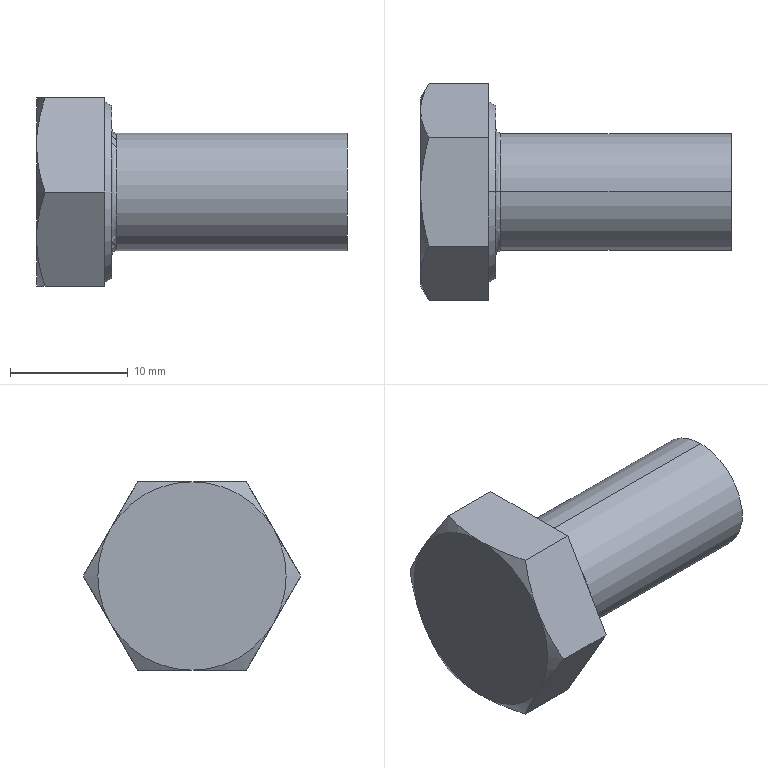Part | SolidWorks | features RevCut 3, Extrusion 1, Fillet 1, LPattern 1, Revolution 1 | 1 solid | 22 faces | box 26.4 x 18.475 x 16 mm | volume 2959 mm3 | plane 10 | cone 8 | torus 2 | cylinder 2 | commonest cylinder face diameters 10 x2
STEP:
#1=CARTESIAN_POINT('',(6.8,0.,5.));
#2=VERTEX_POINT('',#1);
#3=CARTESIAN_POINT('',(6.8,0.,-5.));
#4=VERTEX_POINT('',#3);
#5=CARTESIAN_POINT('',(6.8,0.,0.));
#6=DIRECTION('',(1.,0.,0.));
#7=DIRECTION('',(0.,0.,-1.));
#8=AXIS2_PLACEMENT_3D('',#5,#6,#7);
#9=CIRCLE('',#8,5.);
#10=EDGE_CURVE('',#2,#4,#9,.T.);
#11=ORIENTED_EDGE('',*,*,#10,.F.);
#12=CARTESIAN_POINT('',(6.4,0.,5.4));
#13=VERTEX_POINT('',#12);
#14=CARTESIAN_POINT('',(6.8,0.,5.4));
#15=DIRECTION('',(0.,1.,0.));
#16=DIRECTION('',(0.,0.,1.));
#17=AXIS2_PLACEMENT_3D('',#14,#15,#16);
#18=CIRCLE('',#17,0.4);
#19=EDGE_CURVE('',#2,#13,#18,.T.);
#20=ORIENTED_EDGE('',*,*,#19,.T.);
#21=CARTESIAN_POINT('',(6.4,0.,-5.4));
#22=VERTEX_POINT('',#21);
#23=CARTESIAN_POINT('',(6.4,0.,0.));
#24=DIRECTION('',(-1.,0.,0.));
#25=DIRECTION('',(0.,0.,-1.));
#26=AXIS2_PLACEMENT_3D('',#23,#24,#25);
#27=CIRCLE('',#26,5.4);
#28=EDGE_CURVE('',#22,#13,#27,.T.);
#29=ORIENTED_EDGE('',*,*,#28,.F.);
#30=CARTESIAN_POINT('',(6.8,0.,-5.4));
#31=DIRECTION('',(0.,-1.,0.));
#32=DIRECTION('',(0.,0.,-1.));
#33=AXIS2_PLACEMENT_3D('',#30,#31,#32);
#34=CIRCLE('',#33,0.4);
#35=EDGE_CURVE('',#4,#22,#34,.T.);
#36=ORIENTED_EDGE('',*,*,#35,.F.);
#37=EDGE_LOOP('',(#11,#20,#29,#36));
#38=FACE_OUTER_BOUND('',#37,.T.);
#39=CARTESIAN_POINT('',(6.8,0.,0.));
#40=DIRECTION('',(1.,0.,0.));
#41=DIRECTION('',(0.,0.,-1.));
#42=AXIS2_PLACEMENT_3D('',#39,#40,#41);
#43=TOROIDAL_SURFACE('',#42,5.4,0.4);
#44=ADVANCED_FACE('',(#38),#43,.F.);
#45=CARTESIAN_POINT('',(26.4,0.,5.));
#46=VERTEX_POINT('',#45);
#47=CARTESIAN_POINT('',(26.4,0.,-5.));
#48=VERTEX_POINT('',#47);
#49=CARTESIAN_POINT('',(26.4,0.,0.));
#50=DIRECTION('',(-1.,0.,0.));
#51=DIRECTION('',(0.,0.,1.));
#52=AXIS2_PLACEMENT_3D('',#49,#50,#51);
#53=CIRCLE('',#52,5.);
#54=EDGE_CURVE('',#46,#48,#53,.T.);
#55=ORIENTED_EDGE('',*,*,#54,.T.);
#56=CARTESIAN_POINT('',(0.,0.,-5.));
#57=DIRECTION('',(-1.,0.,0.));
#58=VECTOR('',#57,1000.);
#59=LINE('',#56,#58);
#60=EDGE_CURVE('',#48,#4,#59,.T.);
#61=ORIENTED_EDGE('',*,*,#60,.T.);
#62=CARTESIAN_POINT('',(6.8,0.,0.));
#63=DIRECTION('',(1.,0.,0.));
#64=DIRECTION('',(0.,0.,-1.));
#65=AXIS2_PLACEMENT_3D('',#62,#63,#64);
#66=CIRCLE('',#65,5.);
#67=EDGE_CURVE('',#4,#2,#66,.T.);
#68=ORIENTED_EDGE('',*,*,#67,.T.);
#69=CARTESIAN_POINT('',(0.,0.,5.));
#70=DIRECTION('',(-1.,0.,0.));
#71=VECTOR('',#70,1000.);
#72=LINE('',#69,#71);
#73=EDGE_CURVE('',#46,#2,#72,.T.);
#74=ORIENTED_EDGE('',*,*,#73,.F.);
#75=EDGE_LOOP('',(#55,#61,#68,#74));
#76=FACE_OUTER_BOUND('',#75,.T.);
#77=CARTESIAN_POINT('',(0.,0.,0.));
#78=DIRECTION('',(-1.,0.,0.));
#79=DIRECTION('',(0.,0.,1.));
#80=AXIS2_PLACEMENT_3D('',#77,#78,#79);
#81=CYLINDRICAL_SURFACE('',#80,5.);
#82=ADVANCED_FACE('',(#76),#81,.T.);
#83=CARTESIAN_POINT('',(6.4,0.,7.315));
#84=VERTEX_POINT('',#83);
#85=CARTESIAN_POINT('',(6.4,0.,-7.315));
#86=VERTEX_POINT('',#85);
#87=CARTESIAN_POINT('',(6.4,0.,0.));
#88=DIRECTION('',(-1.,0.,0.));
#89=DIRECTION('',(0.,0.,1.));
#90=AXIS2_PLACEMENT_3D('',#87,#88,#89);
#91=CIRCLE('',#90,7.315);
#92=EDGE_CURVE('',#84,#86,#91,.T.);
#93=ORIENTED_EDGE('',*,*,#92,.T.);
#94=CARTESIAN_POINT('',(5.8,0.,-7.661));
#95=VERTEX_POINT('',#94);
#96=CARTESIAN_POINT('',(5.8,0.,-7.661));
#97=DIRECTION('',(-0.866,0.,-0.5));
#98=VECTOR('',#97,1000.);
#99=LINE('',#96,#98);
#100=EDGE_CURVE('',#86,#95,#99,.T.);
#101=ORIENTED_EDGE('',*,*,#100,.T.);
#102=CARTESIAN_POINT('',(5.8,0.,7.661));
#103=VERTEX_POINT('',#102);
#104=CARTESIAN_POINT('',(5.8,0.,0.));
#105=DIRECTION('',(-1.,0.,0.));
#106=DIRECTION('',(0.,0.,1.));
#107=AXIS2_PLACEMENT_3D('',#104,#105,#106);
#108=CIRCLE('',#107,7.661);
#109=EDGE_CURVE('',#103,#95,#108,.T.);
#110=ORIENTED_EDGE('',*,*,#109,.F.);
#111=CARTESIAN_POINT('',(5.8,0.,7.661));
#112=DIRECTION('',(-0.866,0.,0.5));
#113=VECTOR('',#112,1000.);
#114=LINE('',#111,#113);
#115=EDGE_CURVE('',#84,#103,#114,.T.);
#116=ORIENTED_EDGE('',*,*,#115,.F.);
#117=EDGE_LOOP('',(#93,#101,#110,#116));
#118=FACE_OUTER_BOUND('',#117,.T.);
#119=CARTESIAN_POINT('',(5.8,0.,0.));
#120=DIRECTION('',(-1.,0.,0.));
#121=DIRECTION('',(0.,0.,1.));
#122=AXIS2_PLACEMENT_3D('',#119,#120,#121);
#123=CONICAL_SURFACE('',#122,7.661,0.5236);
#124=ADVANCED_FACE('',(#118),#123,.T.);
#125=CARTESIAN_POINT('',(5.8,4.619,-8.));
#126=VERTEX_POINT('',#125);
#127=CARTESIAN_POINT('',(5.8,9.238,0.));
#128=VERTEX_POINT('',#127);
#129=CARTESIAN_POINT('',(5.8,4.619,-8.));
#130=DIRECTION('',(0.,0.5,0.866));
#131=VECTOR('',#130,1000.);
#132=LINE('',#129,#131);
#133=EDGE_CURVE('',#126,#128,#132,.T.);
#134=ORIENTED_EDGE('',*,*,#133,.F.);
#135=CARTESIAN_POINT('',(0.7145,4.619,-8.));
#136=VERTEX_POINT('',#135);
#137=CARTESIAN_POINT('',(6.4,4.619,-8.));
#138=DIRECTION('',(-1.,0.,0.));
#139=VECTOR('',#138,1000.);
#140=LINE('',#137,#139);
#141=EDGE_CURVE('',#126,#136,#140,.T.);
#142=ORIENTED_EDGE('',*,*,#141,.T.);
#143=CARTESIAN_POINT('',(0.,6.928,-4.));
#144=VERTEX_POINT('',#143);
#145=CARTESIAN_POINT('',(0.,6.928,-4.));
#146=CARTESIAN_POINT('',(0.,6.732,-4.339));
#147=CARTESIAN_POINT('',(0.01689,6.535,-4.68));
#148=CARTESIAN_POINT('',(0.08225,6.146,-5.355));
#149=CARTESIAN_POINT('',(0.1307,5.952,-5.69));
#150=CARTESIAN_POINT('',(0.3174,5.376,-6.689));
#151=CARTESIAN_POINT('',(0.497,4.996,-7.347));
#152=CARTESIAN_POINT('',(0.7145,4.619,-8.));
#153=B_SPLINE_CURVE_WITH_KNOTS('',3,(#145,#146,#147,#148,#149,#150,#151,#152),.UNSPECIFIED.,.F.,.F.,(4,2,2,4),(0.004674,0.005838,0.007002,0.00933),.UNSPECIFIED.);
#154=EDGE_CURVE('',#144,#136,#153,.T.);
#155=ORIENTED_EDGE('',*,*,#154,.F.);
#156=CARTESIAN_POINT('',(0.7145,9.238,0.));
#157=VERTEX_POINT('',#156);
#158=CARTESIAN_POINT('',(0.7145,9.238,0.));
#159=CARTESIAN_POINT('',(0.4964,8.86,-0.6543));
#160=CARTESIAN_POINT('',(0.3167,8.479,-1.313));
#161=CARTESIAN_POINT('',(0.0681,7.71,-2.646));
#162=CARTESIAN_POINT('',(0.,7.322,-3.319));
#163=CARTESIAN_POINT('',(0.,6.928,-4.));
#164=B_SPLINE_CURVE_WITH_KNOTS('',3,(#158,#159,#160,#161,#162,#163),.UNSPECIFIED.,.F.,.F.,(4,2,4),(0.000000238,0.002337,0.004674),.UNSPECIFIED.);
#165=EDGE_CURVE('',#157,#144,#164,.T.);
#166=ORIENTED_EDGE('',*,*,#165,.F.);
#167=CARTESIAN_POINT('',(6.4,9.238,0.));
#168=DIRECTION('',(-1.,0.,0.));
#169=VECTOR('',#168,1000.);
#170=LINE('',#167,#169);
#171=EDGE_CURVE('',#128,#157,#170,.T.);
#172=ORIENTED_EDGE('',*,*,#171,.F.);
#173=EDGE_LOOP('',(#134,#142,#155,#166,#172));
#174=FACE_OUTER_BOUND('',#173,.T.);
#175=CARTESIAN_POINT('',(6.4,4.619,-8.));
#176=DIRECTION('',(0.,-0.866,0.5));
#177=DIRECTION('',(0.,-0.5,-0.866));
#178=AXIS2_PLACEMENT_3D('',#175,#176,#177);
#179=PLANE('',#178);
#180=ADVANCED_FACE('',(#174),#179,.F.);
#181=CARTESIAN_POINT('',(5.8,4.619,8.));
#182=VERTEX_POINT('',#181);
#183=CARTESIAN_POINT('',(5.8,9.238,0.));
#184=DIRECTION('',(0.,-0.5,0.866));
#185=VECTOR('',#184,1000.);
#186=LINE('',#183,#185);
#187=EDGE_CURVE('',#128,#182,#186,.T.);
#188=ORIENTED_EDGE('',*,*,#187,.F.);
#189=ORIENTED_EDGE('',*,*,#171,.T.);
#190=CARTESIAN_POINT('',(0.,6.928,4.));
#191=VERTEX_POINT('',#190);
#192=CARTESIAN_POINT('',(0.,6.928,4.));
#193=CARTESIAN_POINT('',(0.,7.124,3.661));
#194=CARTESIAN_POINT('',(0.01689,7.321,3.32));
#195=CARTESIAN_POINT('',(0.08225,7.711,2.645));
#196=CARTESIAN_POINT('',(0.1307,7.904,2.31));
#197=CARTESIAN_POINT('',(0.3174,8.481,1.311));
#198=CARTESIAN_POINT('',(0.497,8.861,0.6527));
#199=CARTESIAN_POINT('',(0.7145,9.238,0.));
#200=B_SPLINE_CURVE_WITH_KNOTS('',3,(#192,#193,#194,#195,#196,#197,#198,#199),.UNSPECIFIED.,.F.,.F.,(4,2,2,4),(0.004674,0.005838,0.007002,0.00933),.UNSPECIFIED.);
#201=EDGE_CURVE('',#191,#157,#200,.T.);
#202=ORIENTED_EDGE('',*,*,#201,.F.);
#203=CARTESIAN_POINT('',(0.7145,4.619,8.));
#204=VERTEX_POINT('',#203);
#205=CARTESIAN_POINT('',(0.7145,4.619,8.));
#206=CARTESIAN_POINT('',(0.4964,4.997,7.346));
#207=CARTESIAN_POINT('',(0.3167,5.377,6.687));
#208=CARTESIAN_POINT('',(0.0681,6.146,5.354));
#209=CARTESIAN_POINT('',(0.,6.535,4.681));
#210=CARTESIAN_POINT('',(0.,6.928,4.));
#211=B_SPLINE_CURVE_WITH_KNOTS('',3,(#205,#206,#207,#208,#209,#210),.UNSPECIFIED.,.F.,.F.,(4,2,4),(0.000000238,0.002337,0.004674),.UNSPECIFIED.);
#212=EDGE_CURVE('',#204,#191,#211,.T.);
#213=ORIENTED_EDGE('',*,*,#212,.F.);
#214=CARTESIAN_POINT('',(6.4,4.619,8.));
#215=DIRECTION('',(-1.,0.,0.));
#216=VECTOR('',#215,1000.);
#217=LINE('',#214,#216);
#218=EDGE_CURVE('',#182,#204,#217,.T.);
#219=ORIENTED_EDGE('',*,*,#218,.F.);
#220=EDGE_LOOP('',(#188,#189,#202,#213,#219));
#221=FACE_OUTER_BOUND('',#220,.T.);
#222=CARTESIAN_POINT('',(6.4,9.238,0.));
#223=DIRECTION('',(0.,-0.866,-0.5));
#224=DIRECTION('',(0.,0.5,-0.866));
#225=AXIS2_PLACEMENT_3D('',#222,#223,#224);
#226=PLANE('',#225);
#227=ADVANCED_FACE('',(#221),#226,.F.);
#228=CARTESIAN_POINT('',(5.8,-4.619,8.));
#229=VERTEX_POINT('',#228);
#230=CARTESIAN_POINT('',(5.8,4.619,8.));
#231=DIRECTION('',(0.,-1.,0.));
#232=VECTOR('',#231,1000.);
#233=LINE('',#230,#232);
#234=EDGE_CURVE('',#182,#229,#233,.T.);
#235=ORIENTED_EDGE('',*,*,#234,.F.);
#236=ORIENTED_EDGE('',*,*,#218,.T.);
#237=CARTESIAN_POINT('',(0.,0.,8.));
#238=VERTEX_POINT('',#237);
#239=CARTESIAN_POINT('',(0.,0.,8.));
#240=CARTESIAN_POINT('',(0.,0.3913,8.));
#241=CARTESIAN_POINT('',(0.01678,0.7854,8.));
#242=CARTESIAN_POINT('',(0.08286,1.571,8.));
#243=CARTESIAN_POINT('',(0.1318,1.96,8.));
#244=CARTESIAN_POINT('',(0.3194,3.115,8.));
#245=CARTESIAN_POINT('',(0.4988,3.872,8.));
#246=CARTESIAN_POINT('',(0.7145,4.619,8.));
#247=B_SPLINE_CURVE_WITH_KNOTS('',3,(#239,#240,#241,#242,#243,#244,#245,#246),.UNSPECIFIED.,.F.,.F.,(4,2,2,4),(0.01337,0.01454,0.01571,0.01805),.UNSPECIFIED.);
#248=EDGE_CURVE('',#238,#204,#247,.T.);
#249=ORIENTED_EDGE('',*,*,#248,.F.);
#250=CARTESIAN_POINT('',(0.7145,-4.619,8.));
#251=VERTEX_POINT('',#250);
#252=CARTESIAN_POINT('',(0.7145,-4.619,8.));
#253=CARTESIAN_POINT('',(0.4973,-3.866,8.));
#254=CARTESIAN_POINT('',(0.3158,-3.098,8.));
#255=CARTESIAN_POINT('',(0.0673,-1.557,8.));
#256=CARTESIAN_POINT('',(0.,-0.7819,8.));
#257=CARTESIAN_POINT('',(0.,0.,8.));
#258=B_SPLINE_CURVE_WITH_KNOTS('',3,(#252,#253,#254,#255,#256,#257),.UNSPECIFIED.,.F.,.F.,(4,2,4),(0.00869,0.01103,0.01337),.UNSPECIFIED.);
#259=EDGE_CURVE('',#251,#238,#258,.T.);
#260=ORIENTED_EDGE('',*,*,#259,.F.);
#261=CARTESIAN_POINT('',(6.4,-4.619,8.));
#262=DIRECTION('',(-1.,0.,0.));
#263=VECTOR('',#262,1000.);
#264=LINE('',#261,#263);
#265=EDGE_CURVE('',#229,#251,#264,.T.);
#266=ORIENTED_EDGE('',*,*,#265,.F.);
#267=EDGE_LOOP('',(#235,#236,#249,#260,#266));
#268=FACE_OUTER_BOUND('',#267,.T.);
#269=CARTESIAN_POINT('',(6.4,4.619,8.));
#270=DIRECTION('',(0.,0.,-1.));
#271=DIRECTION('',(0.,1.,0.));
#272=AXIS2_PLACEMENT_3D('',#269,#270,#271);
#273=PLANE('',#272);
#274=ADVANCED_FACE('',(#268),#273,.F.);
#275=CARTESIAN_POINT('',(5.8,-9.238,0.));
#276=VERTEX_POINT('',#275);
#277=CARTESIAN_POINT('',(5.8,-9.238,0.));
#278=DIRECTION('',(0.,-0.5,-0.866));
#279=VECTOR('',#278,1000.);
#280=LINE('',#277,#279);
#281=EDGE_CURVE('',#229,#276,#280,.T.);
#282=ORIENTED_EDGE('',*,*,#281,.F.);
#283=ORIENTED_EDGE('',*,*,#265,.T.);
#284=CARTESIAN_POINT('',(0.,-6.928,4.));
#285=VERTEX_POINT('',#284);
#286=CARTESIAN_POINT('',(0.,-6.928,4.));
#287=CARTESIAN_POINT('',(0.,-6.732,4.339));
#288=CARTESIAN_POINT('',(0.01689,-6.535,4.68));
#289=CARTESIAN_POINT('',(0.08225,-6.146,5.355));
#290=CARTESIAN_POINT('',(0.1307,-5.952,5.69));
#291=CARTESIAN_POINT('',(0.3174,-5.376,6.689));
#292=CARTESIAN_POINT('',(0.497,-4.996,7.347));
#293=CARTESIAN_POINT('',(0.7145,-4.619,8.));
#294=B_SPLINE_CURVE_WITH_KNOTS('',3,(#286,#287,#288,#289,#290,#291,#292,#293),.UNSPECIFIED.,.F.,.F.,(4,2,2,4),(0.004674,0.005838,0.007002,0.00933),.UNSPECIFIED.);
#295=EDGE_CURVE('',#285,#251,#294,.T.);
#296=ORIENTED_EDGE('',*,*,#295,.F.);
#297=CARTESIAN_POINT('',(0.7145,-9.238,0.));
#298=VERTEX_POINT('',#297);
#299=CARTESIAN_POINT('',(0.7145,-9.238,0.));
#300=CARTESIAN_POINT('',(0.4964,-8.86,0.6543));
#301=CARTESIAN_POINT('',(0.3167,-8.479,1.313));
#302=CARTESIAN_POINT('',(0.0681,-7.71,2.646));
#303=CARTESIAN_POINT('',(0.,-7.322,3.319));
#304=CARTESIAN_POINT('',(0.,-6.928,4.));
#305=B_SPLINE_CURVE_WITH_KNOTS('',3,(#299,#300,#301,#302,#303,#304),.UNSPECIFIED.,.F.,.F.,(4,2,4),(0.000000238,0.002337,0.004674),.UNSPECIFIED.);
#306=EDGE_CURVE('',#298,#285,#305,.T.);
#307=ORIENTED_EDGE('',*,*,#306,.F.);
#308=CARTESIAN_POINT('',(6.4,-9.238,0.));
#309=DIRECTION('',(-1.,0.,0.));
#310=VECTOR('',#309,1000.);
#311=LINE('',#308,#310);
#312=EDGE_CURVE('',#276,#298,#311,.T.);
#313=ORIENTED_EDGE('',*,*,#312,.F.);
#314=EDGE_LOOP('',(#282,#283,#296,#307,#313));
#315=FACE_OUTER_BOUND('',#314,.T.);
#316=CARTESIAN_POINT('',(6.4,-9.238,0.));
#317=DIRECTION('',(0.,0.866,-0.5));
#318=DIRECTION('',(0.,0.5,0.866));
#319=AXIS2_PLACEMENT_3D('',#316,#317,#318);
#320=PLANE('',#319);
#321=ADVANCED_FACE('',(#315),#320,.F.);
#322=CARTESIAN_POINT('',(5.8,-4.619,-8.));
#323=VERTEX_POINT('',#322);
#324=CARTESIAN_POINT('',(5.8,-4.619,-8.));
#325=DIRECTION('',(0.,0.5,-0.866));
#326=VECTOR('',#325,1000.);
#327=LINE('',#324,#326);
#328=EDGE_CURVE('',#276,#323,#327,.T.);
#329=ORIENTED_EDGE('',*,*,#328,.F.);
#330=ORIENTED_EDGE('',*,*,#312,.T.);
#331=CARTESIAN_POINT('',(0.,-6.928,-4.));
#332=VERTEX_POINT('',#331);
#333=CARTESIAN_POINT('',(0.,-6.928,-4.));
#334=CARTESIAN_POINT('',(0.,-7.124,-3.661));
#335=CARTESIAN_POINT('',(0.01689,-7.321,-3.32));
#336=CARTESIAN_POINT('',(0.08225,-7.711,-2.645));
#337=CARTESIAN_POINT('',(0.1307,-7.904,-2.31));
#338=CARTESIAN_POINT('',(0.3174,-8.481,-1.311));
#339=CARTESIAN_POINT('',(0.497,-8.861,-0.6527));
#340=CARTESIAN_POINT('',(0.7145,-9.238,0.));
#341=B_SPLINE_CURVE_WITH_KNOTS('',3,(#333,#334,#335,#336,#337,#338,#339,#340),.UNSPECIFIED.,.F.,.F.,(4,2,2,4),(0.004674,0.005838,0.007002,0.00933),.UNSPECIFIED.);
#342=EDGE_CURVE('',#332,#298,#341,.T.);
#343=ORIENTED_EDGE('',*,*,#342,.F.);
#344=CARTESIAN_POINT('',(0.7145,-4.619,-8.));
#345=VERTEX_POINT('',#344);
#346=CARTESIAN_POINT('',(0.7145,-4.619,-8.));
#347=CARTESIAN_POINT('',(0.4964,-4.997,-7.346));
#348=CARTESIAN_POINT('',(0.3167,-5.377,-6.687));
#349=CARTESIAN_POINT('',(0.0681,-6.146,-5.354));
#350=CARTESIAN_POINT('',(0.,-6.535,-4.681));
#351=CARTESIAN_POINT('',(0.,-6.928,-4.));
#352=B_SPLINE_CURVE_WITH_KNOTS('',3,(#346,#347,#348,#349,#350,#351),.UNSPECIFIED.,.F.,.F.,(4,2,4),(0.000000238,0.002337,0.004674),.UNSPECIFIED.);
#353=EDGE_CURVE('',#345,#332,#352,.T.);
#354=ORIENTED_EDGE('',*,*,#353,.F.);
#355=CARTESIAN_POINT('',(6.4,-4.619,-8.));
#356=DIRECTION('',(-1.,0.,0.));
#357=VECTOR('',#356,1000.);
#358=LINE('',#355,#357);
#359=EDGE_CURVE('',#323,#345,#358,.T.);
#360=ORIENTED_EDGE('',*,*,#359,.F.);
#361=EDGE_LOOP('',(#329,#330,#343,#354,#360));
#362=FACE_OUTER_BOUND('',#361,.T.);
#363=CARTESIAN_POINT('',(6.4,-4.619,-8.));
#364=DIRECTION('',(0.,0.866,0.5));
#365=DIRECTION('',(0.,-0.5,0.866));
#366=AXIS2_PLACEMENT_3D('',#363,#364,#365);
#367=PLANE('',#366);
#368=ADVANCED_FACE('',(#362),#367,.F.);
#369=CARTESIAN_POINT('',(5.8,4.619,-8.));
#370=DIRECTION('',(0.,1.,0.));
#371=VECTOR('',#370,1000.);
#372=LINE('',#369,#371);
#373=EDGE_CURVE('',#323,#126,#372,.T.);
#374=ORIENTED_EDGE('',*,*,#373,.F.);
#375=ORIENTED_EDGE('',*,*,#359,.T.);
#376=CARTESIAN_POINT('',(0.,0.,-8.));
#377=VERTEX_POINT('',#376);
#378=CARTESIAN_POINT('',(0.,0.,-8.));
#379=CARTESIAN_POINT('',(0.,-0.7819,-8.));
#380=CARTESIAN_POINT('',(0.0673,-1.557,-8.));
#381=CARTESIAN_POINT('',(0.3158,-3.098,-8.));
#382=CARTESIAN_POINT('',(0.4973,-3.866,-8.));
#383=CARTESIAN_POINT('',(0.7145,-4.619,-8.));
#384=B_SPLINE_CURVE_WITH_KNOTS('',3,(#378,#379,#380,#381,#382,#383),.UNSPECIFIED.,.F.,.F.,(4,2,4),(0.02753,0.02987,0.03221),.UNSPECIFIED.);
#385=EDGE_CURVE('',#377,#345,#384,.T.);
#386=ORIENTED_EDGE('',*,*,#385,.F.);
#387=CARTESIAN_POINT('',(0.7145,4.619,-8.));
#388=CARTESIAN_POINT('',(0.4988,3.872,-8.));
#389=CARTESIAN_POINT('',(0.3194,3.115,-8.));
#390=CARTESIAN_POINT('',(0.1318,1.96,-8.));
#391=CARTESIAN_POINT('',(0.08286,1.571,-8.));
#392=CARTESIAN_POINT('',(0.01678,0.7854,-8.));
#393=CARTESIAN_POINT('',(0.,0.3913,-8.));
#394=CARTESIAN_POINT('',(0.,0.,-8.));
#395=B_SPLINE_CURVE_WITH_KNOTS('',3,(#387,#388,#389,#390,#391,#392,#393,#394),.UNSPECIFIED.,.F.,.F.,(4,2,2,4),(0.02285,0.02519,0.02636,0.02753),.UNSPECIFIED.);
#396=EDGE_CURVE('',#136,#377,#395,.T.);
#397=ORIENTED_EDGE('',*,*,#396,.F.);
#398=ORIENTED_EDGE('',*,*,#141,.F.);
#399=EDGE_LOOP('',(#374,#375,#386,#397,#398));
#400=FACE_OUTER_BOUND('',#399,.T.);
#401=CARTESIAN_POINT('',(6.4,4.619,-8.));
#402=DIRECTION('',(0.,0.,1.));
#403=DIRECTION('',(1.,0.,0.));
#404=AXIS2_PLACEMENT_3D('',#401,#402,#403);
#405=PLANE('',#404);
#406=ADVANCED_FACE('',(#400),#405,.F.);
#407=ORIENTED_EDGE('',*,*,#353,.T.);
#408=CARTESIAN_POINT('',(0.,0.,0.));
#409=DIRECTION('',(1.,0.,0.));
#410=DIRECTION('',(0.,0.,-1.));
#411=AXIS2_PLACEMENT_3D('',#408,#409,#410);
#412=CIRCLE('',#411,8.);
#413=EDGE_CURVE('',#332,#377,#412,.T.);
#414=ORIENTED_EDGE('',*,*,#413,.T.);
#415=ORIENTED_EDGE('',*,*,#385,.T.);
#416=EDGE_LOOP('',(#407,#414,#415));
#417=FACE_OUTER_BOUND('',#416,.T.);
#418=CARTESIAN_POINT('',(0.,0.,0.));
#419=DIRECTION('',(1.,0.,0.));
#420=DIRECTION('',(0.,0.,-1.));
#421=AXIS2_PLACEMENT_3D('',#418,#419,#420);
#422=CONICAL_SURFACE('',#421,8.,1.047);
#423=ADVANCED_FACE('',(#417),#422,.T.);
#424=ORIENTED_EDGE('',*,*,#306,.T.);
#425=CARTESIAN_POINT('',(0.,0.,0.));
#426=DIRECTION('',(1.,0.,0.));
#427=DIRECTION('',(0.,0.,-1.));
#428=AXIS2_PLACEMENT_3D('',#425,#426,#427);
#429=CIRCLE('',#428,8.);
#430=EDGE_CURVE('',#285,#332,#429,.T.);
#431=ORIENTED_EDGE('',*,*,#430,.T.);
#432=ORIENTED_EDGE('',*,*,#342,.T.);
#433=EDGE_LOOP('',(#424,#431,#432));
#434=FACE_OUTER_BOUND('',#433,.T.);
#435=CARTESIAN_POINT('',(0.,0.,0.));
#436=DIRECTION('',(1.,0.,0.));
#437=DIRECTION('',(0.,0.,-1.));
#438=AXIS2_PLACEMENT_3D('',#435,#436,#437);
#439=CONICAL_SURFACE('',#438,8.,1.047);
#440=ADVANCED_FACE('',(#434),#439,.T.);
#441=ORIENTED_EDGE('',*,*,#259,.T.);
#442=CARTESIAN_POINT('',(0.,0.,0.));
#443=DIRECTION('',(1.,0.,0.));
#444=DIRECTION('',(0.,0.,-1.));
#445=AXIS2_PLACEMENT_3D('',#442,#443,#444);
#446=CIRCLE('',#445,8.);
#447=EDGE_CURVE('',#238,#285,#446,.T.);
#448=ORIENTED_EDGE('',*,*,#447,.T.);
#449=ORIENTED_EDGE('',*,*,#295,.T.);
#450=EDGE_LOOP('',(#441,#448,#449));
#451=FACE_OUTER_BOUND('',#450,.T.);
#452=CARTESIAN_POINT('',(0.,0.,0.));
#453=DIRECTION('',(1.,0.,0.));
#454=DIRECTION('',(0.,0.,-1.));
#455=AXIS2_PLACEMENT_3D('',#452,#453,#454);
#456=CONICAL_SURFACE('',#455,8.,1.047);
#457=ADVANCED_FACE('',(#451),#456,.T.);
#458=ORIENTED_EDGE('',*,*,#248,.T.);
#459=ORIENTED_EDGE('',*,*,#212,.T.);
#460=CARTESIAN_POINT('',(0.,0.,0.));
#461=DIRECTION('',(-1.,0.,0.));
#462=DIRECTION('',(0.,0.,1.));
#463=AXIS2_PLACEMENT_3D('',#460,#461,#462);
#464=CIRCLE('',#463,8.);
#465=EDGE_CURVE('',#238,#191,#464,.T.);
#466=ORIENTED_EDGE('',*,*,#465,.F.);
#467=EDGE_LOOP('',(#458,#459,#466));
#468=FACE_OUTER_BOUND('',#467,.T.);
#469=CARTESIAN_POINT('',(0.,0.,0.));
#470=DIRECTION('',(1.,0.,0.));
#471=DIRECTION('',(0.,0.,-1.));
#472=AXIS2_PLACEMENT_3D('',#469,#470,#471);
#473=CONICAL_SURFACE('',#472,8.,1.047);
#474=ADVANCED_FACE('',(#468),#473,.T.);
#475=ORIENTED_EDGE('',*,*,#201,.T.);
#476=ORIENTED_EDGE('',*,*,#165,.T.);
#477=CARTESIAN_POINT('',(0.,0.,0.));
#478=DIRECTION('',(1.,0.,0.));
#479=DIRECTION('',(0.,0.,-1.));
#480=AXIS2_PLACEMENT_3D('',#477,#478,#479);
#481=CIRCLE('',#480,8.);
#482=EDGE_CURVE('',#144,#191,#481,.T.);
#483=ORIENTED_EDGE('',*,*,#482,.T.);
#484=EDGE_LOOP('',(#475,#476,#483));
#485=FACE_OUTER_BOUND('',#484,.T.);
#486=CARTESIAN_POINT('',(0.,0.,0.));
#487=DIRECTION('',(1.,0.,0.));
#488=DIRECTION('',(0.,0.,-1.));
#489=AXIS2_PLACEMENT_3D('',#486,#487,#488);
#490=CONICAL_SURFACE('',#489,8.,1.047);
#491=ADVANCED_FACE('',(#485),#490,.T.);
#492=ORIENTED_EDGE('',*,*,#154,.T.);
#493=ORIENTED_EDGE('',*,*,#396,.T.);
#494=CARTESIAN_POINT('',(0.,0.,0.));
#495=DIRECTION('',(1.,0.,0.));
#496=DIRECTION('',(0.,0.,-1.));
#497=AXIS2_PLACEMENT_3D('',#494,#495,#496);
#498=CIRCLE('',#497,8.);
#499=EDGE_CURVE('',#377,#144,#498,.T.);
#500=ORIENTED_EDGE('',*,*,#499,.T.);
#501=EDGE_LOOP('',(#492,#493,#500));
#502=FACE_OUTER_BOUND('',#501,.T.);
#503=CARTESIAN_POINT('',(0.,0.,0.));
#504=DIRECTION('',(1.,0.,0.));
#505=DIRECTION('',(0.,0.,-1.));
#506=AXIS2_PLACEMENT_3D('',#503,#504,#505);
#507=CONICAL_SURFACE('',#506,8.,1.047);
#508=ADVANCED_FACE('',(#502),#507,.T.);
#509=ORIENTED_EDGE('',*,*,#499,.F.);
#510=ORIENTED_EDGE('',*,*,#413,.F.);
#511=ORIENTED_EDGE('',*,*,#430,.F.);
#512=ORIENTED_EDGE('',*,*,#447,.F.);
#513=ORIENTED_EDGE('',*,*,#465,.T.);
#514=ORIENTED_EDGE('',*,*,#482,.F.);
#515=EDGE_LOOP('',(#509,#510,#511,#512,#513,#514));
#516=FACE_OUTER_BOUND('',#515,.T.);
#517=CARTESIAN_POINT('',(0.,9.238,0.));
#518=DIRECTION('',(1.,0.,0.));
#519=DIRECTION('',(0.,0.,-1.));
#520=AXIS2_PLACEMENT_3D('',#517,#518,#519);
#521=PLANE('',#520);
#522=ADVANCED_FACE('',(#516),#521,.F.);
#523=ORIENTED_EDGE('',*,*,#109,.T.);
#524=CARTESIAN_POINT('',(5.8,0.,0.));
#525=DIRECTION('',(-1.,0.,0.));
#526=DIRECTION('',(0.,0.,1.));
#527=AXIS2_PLACEMENT_3D('',#524,#525,#526);
#528=CIRCLE('',#527,7.661);
#529=EDGE_CURVE('',#95,#103,#528,.T.);
#530=ORIENTED_EDGE('',*,*,#529,.T.);
#531=EDGE_LOOP('',(#523,#530));
#532=FACE_BOUND('',#531,.T.);
#533=ORIENTED_EDGE('',*,*,#133,.T.);
#534=ORIENTED_EDGE('',*,*,#187,.T.);
#535=ORIENTED_EDGE('',*,*,#234,.T.);
#536=ORIENTED_EDGE('',*,*,#281,.T.);
#537=ORIENTED_EDGE('',*,*,#328,.T.);
#538=ORIENTED_EDGE('',*,*,#373,.T.);
#539=EDGE_LOOP('',(#533,#534,#535,#536,#537,#538));
#540=FACE_OUTER_BOUND('',#539,.T.);
#541=CARTESIAN_POINT('',(5.8,7.661,0.));
#542=DIRECTION('',(1.,0.,0.));
#543=DIRECTION('',(0.,0.,-1.));
#544=AXIS2_PLACEMENT_3D('',#541,#542,#543);
#545=PLANE('',#544);
#546=ADVANCED_FACE('',(#532,#540),#545,.T.);
#547=ORIENTED_EDGE('',*,*,#100,.F.);
#548=CARTESIAN_POINT('',(6.4,0.,0.));
#549=DIRECTION('',(-1.,0.,0.));
#550=DIRECTION('',(0.,0.,1.));
#551=AXIS2_PLACEMENT_3D('',#548,#549,#550);
#552=CIRCLE('',#551,7.315);
#553=EDGE_CURVE('',#86,#84,#552,.T.);
#554=ORIENTED_EDGE('',*,*,#553,.T.);
#555=ORIENTED_EDGE('',*,*,#115,.T.);
#556=ORIENTED_EDGE('',*,*,#529,.F.);
#557=EDGE_LOOP('',(#547,#554,#555,#556));
#558=FACE_OUTER_BOUND('',#557,.T.);
#559=CARTESIAN_POINT('',(5.8,0.,0.));
#560=DIRECTION('',(-1.,0.,0.));
#561=DIRECTION('',(0.,0.,1.));
#562=AXIS2_PLACEMENT_3D('',#559,#560,#561);
#563=CONICAL_SURFACE('',#562,7.661,0.5236);
#564=ADVANCED_FACE('',(#558),#563,.T.);
#565=ORIENTED_EDGE('',*,*,#54,.F.);
#566=CARTESIAN_POINT('',(26.4,0.,0.));
#567=DIRECTION('',(-1.,0.,0.));
#568=DIRECTION('',(0.,0.,1.));
#569=AXIS2_PLACEMENT_3D('',#566,#567,#568);
#570=CIRCLE('',#569,5.);
#571=EDGE_CURVE('',#48,#46,#570,.T.);
#572=ORIENTED_EDGE('',*,*,#571,.F.);
#573=EDGE_LOOP('',(#565,#572));
#574=FACE_OUTER_BOUND('',#573,.T.);
#575=CARTESIAN_POINT('',(26.4,0.,0.));
#576=DIRECTION('',(-1.,0.,0.));
#577=DIRECTION('',(0.,0.,1.));
#578=AXIS2_PLACEMENT_3D('',#575,#576,#577);
#579=PLANE('',#578);
#580=ADVANCED_FACE('',(#574),#579,.F.);
#581=ORIENTED_EDGE('',*,*,#60,.F.);
#582=ORIENTED_EDGE('',*,*,#571,.T.);
#583=ORIENTED_EDGE('',*,*,#73,.T.);
#584=ORIENTED_EDGE('',*,*,#10,.T.);
#585=EDGE_LOOP('',(#581,#582,#583,#584));
#586=FACE_OUTER_BOUND('',#585,.T.);
#587=CARTESIAN_POINT('',(0.,0.,0.));
#588=DIRECTION('',(-1.,0.,0.));
#589=DIRECTION('',(0.,0.,1.));
#590=AXIS2_PLACEMENT_3D('',#587,#588,#589);
#591=CYLINDRICAL_SURFACE('',#590,5.);
#592=ADVANCED_FACE('',(#586),#591,.T.);
#593=ORIENTED_EDGE('',*,*,#28,.T.);
#594=CARTESIAN_POINT('',(6.4,0.,0.));
#595=DIRECTION('',(-1.,0.,0.));
#596=DIRECTION('',(0.,0.,-1.));
#597=AXIS2_PLACEMENT_3D('',#594,#595,#596);
#598=CIRCLE('',#597,5.4);
#599=EDGE_CURVE('',#13,#22,#598,.T.);
#600=ORIENTED_EDGE('',*,*,#599,.T.);
#601=EDGE_LOOP('',(#593,#600));
#602=FACE_BOUND('',#601,.T.);
#603=ORIENTED_EDGE('',*,*,#92,.F.);
#604=ORIENTED_EDGE('',*,*,#553,.F.);
#605=EDGE_LOOP('',(#603,#604));
#606=FACE_OUTER_BOUND('',#605,.T.);
#607=CARTESIAN_POINT('',(6.4,9.238,0.));
#608=DIRECTION('',(1.,0.,0.));
#609=DIRECTION('',(0.,0.,-1.));
#610=AXIS2_PLACEMENT_3D('',#607,#608,#609);
#611=PLANE('',#610);
#612=ADVANCED_FACE('',(#602,#606),#611,.T.);
#613=ORIENTED_EDGE('',*,*,#19,.F.);
#614=ORIENTED_EDGE('',*,*,#67,.F.);
#615=ORIENTED_EDGE('',*,*,#35,.T.);
#616=ORIENTED_EDGE('',*,*,#599,.F.);
#617=EDGE_LOOP('',(#613,#614,#615,#616));
#618=FACE_OUTER_BOUND('',#617,.T.);
#619=CARTESIAN_POINT('',(6.8,0.,0.));
#620=DIRECTION('',(1.,0.,0.));
#621=DIRECTION('',(0.,0.,-1.));
#622=AXIS2_PLACEMENT_3D('',#619,#620,#621);
#623=TOROIDAL_SURFACE('',#622,5.4,0.4);
#624=ADVANCED_FACE('',(#618),#623,.F.);
#625=CLOSED_SHELL('',(#44,#82,#124,#180,#227,#274,#321,#368,#406,#423,#440,#457,#474,#491,#508,#522,#546,#564,#580,#592,#612,#624));
#626=MANIFOLD_SOLID_BREP('',#625);
#627=CARTESIAN_POINT('',(0.,0.,0.));
#628=DIRECTION('',(0.,0.,1.));
#629=DIRECTION('',(1.,0.,0.));
#630=AXIS2_PLACEMENT_3D('',#627,#628,#629);
#631=(LENGTH_UNIT()NAMED_UNIT(*)SI_UNIT(.MILLI.,.METRE.));
#632=UNCERTAINTY_MEASURE_WITH_UNIT(LENGTH_MEASURE(0.00001),#631,'','');
#633=(NAMED_UNIT(*)PLANE_ANGLE_UNIT()SI_UNIT($,.RADIAN.));
#634=(NAMED_UNIT(*)SI_UNIT($,.STERADIAN.)SOLID_ANGLE_UNIT());
#635=(GEOMETRIC_REPRESENTATION_CONTEXT(3)GLOBAL_UNCERTAINTY_ASSIGNED_CONTEXT((#632))GLOBAL_UNIT_ASSIGNED_CONTEXT((#631,#633,#634))REPRESENTATION_CONTEXT('',''));
#636=ADVANCED_BREP_SHAPE_REPRESENTATION('',(#626,#630),#635);